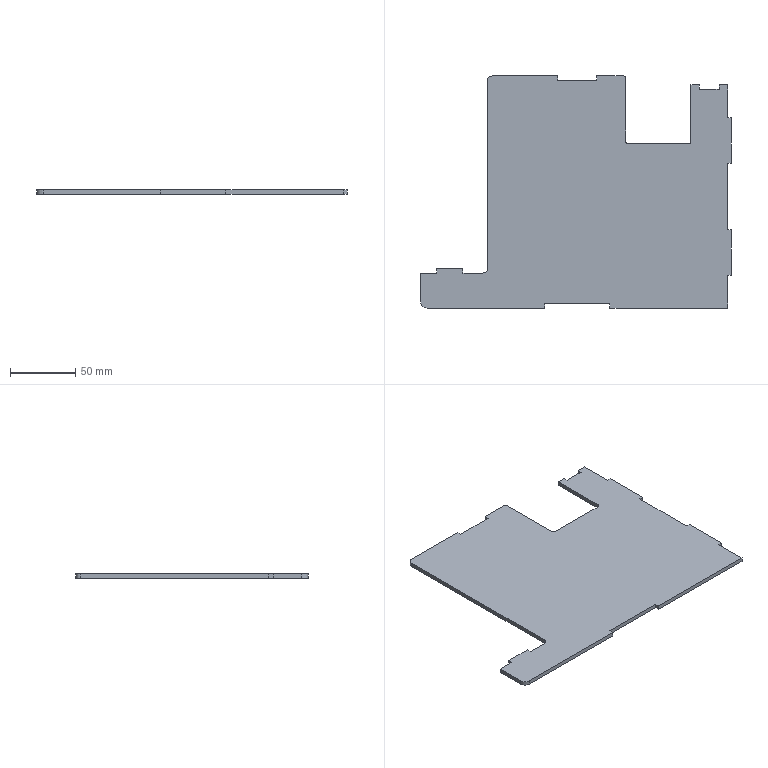Part | SolidWorks | features FlatPattern 1, SMBaseFlange 1, SheetMetal 1 | 1 solid | 42 faces | box 238 x 177.7 x 3.2 mm | volume 99826 mm3 | plane 36 | cylinder 6 | commonest cylinder face diameters 4 x3 7 x2 10 x1
STEP:
#1=CARTESIAN_POINT('',(12.5,-5.5,0.));
#2=VERTEX_POINT('',#1);
#3=CARTESIAN_POINT('',(0.,-5.5,0.));
#4=VERTEX_POINT('',#3);
#5=CARTESIAN_POINT('',(12.5,-5.5,0.));
#6=DIRECTION('',(-1.,0.,0.));
#7=VECTOR('',#6,1000.);
#8=LINE('',#5,#7);
#9=EDGE_CURVE('',#2,#4,#8,.T.);
#10=ORIENTED_EDGE('',*,*,#9,.F.);
#11=CARTESIAN_POINT('',(12.5,-5.5,-3.2));
#12=VERTEX_POINT('',#11);
#13=CARTESIAN_POINT('',(12.5,-5.5,-3.2));
#14=DIRECTION('',(0.,0.,1.));
#15=VECTOR('',#14,1000.);
#16=LINE('',#13,#15);
#17=EDGE_CURVE('',#12,#2,#16,.T.);
#18=ORIENTED_EDGE('',*,*,#17,.F.);
#19=CARTESIAN_POINT('',(0.,-5.5,-3.2));
#20=VERTEX_POINT('',#19);
#21=CARTESIAN_POINT('',(12.5,-5.5,-3.2));
#22=DIRECTION('',(-1.,0.,0.));
#23=VECTOR('',#22,1000.);
#24=LINE('',#21,#23);
#25=EDGE_CURVE('',#12,#20,#24,.T.);
#26=ORIENTED_EDGE('',*,*,#25,.T.);
#27=CARTESIAN_POINT('',(0.,-5.5,-3.2));
#28=DIRECTION('',(0.,0.,1.));
#29=VECTOR('',#28,1000.);
#30=LINE('',#27,#29);
#31=EDGE_CURVE('',#20,#4,#30,.T.);
#32=ORIENTED_EDGE('',*,*,#31,.T.);
#33=EDGE_LOOP('',(#10,#18,#26,#32));
#34=FACE_OUTER_BOUND('',#33,.T.);
#35=CARTESIAN_POINT('',(12.5,-5.5,-3.2));
#36=DIRECTION('',(0.,1.,0.));
#37=DIRECTION('',(-1.,0.,0.));
#38=AXIS2_PLACEMENT_3D('',#35,#36,#37);
#39=PLANE('',#38);
#40=ADVANCED_FACE('',(#34),#39,.T.);
#41=CARTESIAN_POINT('',(12.5,-2.3,0.));
#42=VERTEX_POINT('',#41);
#43=CARTESIAN_POINT('',(12.5,-5.5,0.));
#44=DIRECTION('',(0.,-1.,0.));
#45=VECTOR('',#44,1000.);
#46=LINE('',#43,#45);
#47=EDGE_CURVE('',#42,#2,#46,.T.);
#48=ORIENTED_EDGE('',*,*,#47,.F.);
#49=CARTESIAN_POINT('',(12.5,-2.3,-3.2));
#50=VERTEX_POINT('',#49);
#51=CARTESIAN_POINT('',(12.5,-2.3,-3.2));
#52=DIRECTION('',(0.,0.,1.));
#53=VECTOR('',#52,1000.);
#54=LINE('',#51,#53);
#55=EDGE_CURVE('',#50,#42,#54,.T.);
#56=ORIENTED_EDGE('',*,*,#55,.F.);
#57=CARTESIAN_POINT('',(12.5,-5.5,-3.2));
#58=DIRECTION('',(0.,-1.,0.));
#59=VECTOR('',#58,1000.);
#60=LINE('',#57,#59);
#61=EDGE_CURVE('',#50,#12,#60,.T.);
#62=ORIENTED_EDGE('',*,*,#61,.T.);
#63=ORIENTED_EDGE('',*,*,#17,.T.);
#64=EDGE_LOOP('',(#48,#56,#62,#63));
#65=FACE_OUTER_BOUND('',#64,.T.);
#66=CARTESIAN_POINT('',(12.5,-5.5,-3.2));
#67=DIRECTION('',(-1.,0.,0.));
#68=DIRECTION('',(0.,0.,1.));
#69=AXIS2_PLACEMENT_3D('',#66,#67,#68);
#70=PLANE('',#69);
#71=ADVANCED_FACE('',(#65),#70,.T.);
#72=CARTESIAN_POINT('',(32.5,-2.3,0.));
#73=VERTEX_POINT('',#72);
#74=CARTESIAN_POINT('',(12.5,-2.3,0.));
#75=DIRECTION('',(-1.,0.,0.));
#76=VECTOR('',#75,1000.);
#77=LINE('',#74,#76);
#78=EDGE_CURVE('',#73,#42,#77,.T.);
#79=ORIENTED_EDGE('',*,*,#78,.F.);
#80=CARTESIAN_POINT('',(32.5,-2.3,-3.2));
#81=VERTEX_POINT('',#80);
#82=CARTESIAN_POINT('',(32.5,-2.3,-3.2));
#83=DIRECTION('',(0.,0.,1.));
#84=VECTOR('',#83,1000.);
#85=LINE('',#82,#84);
#86=EDGE_CURVE('',#81,#73,#85,.T.);
#87=ORIENTED_EDGE('',*,*,#86,.F.);
#88=CARTESIAN_POINT('',(12.5,-2.3,-3.2));
#89=DIRECTION('',(-1.,0.,0.));
#90=VECTOR('',#89,1000.);
#91=LINE('',#88,#90);
#92=EDGE_CURVE('',#81,#50,#91,.T.);
#93=ORIENTED_EDGE('',*,*,#92,.T.);
#94=ORIENTED_EDGE('',*,*,#55,.T.);
#95=EDGE_LOOP('',(#79,#87,#93,#94));
#96=FACE_OUTER_BOUND('',#95,.T.);
#97=CARTESIAN_POINT('',(12.5,-2.3,-3.2));
#98=DIRECTION('',(0.,1.,0.));
#99=DIRECTION('',(0.,0.,1.));
#100=AXIS2_PLACEMENT_3D('',#97,#98,#99);
#101=PLANE('',#100);
#102=ADVANCED_FACE('',(#96),#101,.T.);
#103=CARTESIAN_POINT('',(32.5,-5.5,0.));
#104=VERTEX_POINT('',#103);
#105=CARTESIAN_POINT('',(32.5,-2.3,0.));
#106=DIRECTION('',(0.,1.,0.));
#107=VECTOR('',#106,1000.);
#108=LINE('',#105,#107);
#109=EDGE_CURVE('',#104,#73,#108,.T.);
#110=ORIENTED_EDGE('',*,*,#109,.F.);
#111=CARTESIAN_POINT('',(32.5,-5.5,-3.2));
#112=VERTEX_POINT('',#111);
#113=CARTESIAN_POINT('',(32.5,-5.5,-3.2));
#114=DIRECTION('',(0.,0.,1.));
#115=VECTOR('',#114,1000.);
#116=LINE('',#113,#115);
#117=EDGE_CURVE('',#112,#104,#116,.T.);
#118=ORIENTED_EDGE('',*,*,#117,.F.);
#119=CARTESIAN_POINT('',(32.5,-2.3,-3.2));
#120=DIRECTION('',(0.,1.,0.));
#121=VECTOR('',#120,1000.);
#122=LINE('',#119,#121);
#123=EDGE_CURVE('',#112,#81,#122,.T.);
#124=ORIENTED_EDGE('',*,*,#123,.T.);
#125=ORIENTED_EDGE('',*,*,#86,.T.);
#126=EDGE_LOOP('',(#110,#118,#124,#125));
#127=FACE_OUTER_BOUND('',#126,.T.);
#128=CARTESIAN_POINT('',(32.5,-2.3,-3.2));
#129=DIRECTION('',(1.,0.,0.));
#130=DIRECTION('',(0.,0.,-1.));
#131=AXIS2_PLACEMENT_3D('',#128,#129,#130);
#132=PLANE('',#131);
#133=ADVANCED_FACE('',(#127),#132,.T.);
#134=CARTESIAN_POINT('',(47.8,-5.5,0.));
#135=VERTEX_POINT('',#134);
#136=CARTESIAN_POINT('',(47.8,-5.5,0.));
#137=DIRECTION('',(-1.,0.,0.));
#138=VECTOR('',#137,1000.);
#139=LINE('',#136,#138);
#140=EDGE_CURVE('',#135,#104,#139,.T.);
#141=ORIENTED_EDGE('',*,*,#140,.F.);
#142=CARTESIAN_POINT('',(47.8,-5.5,-3.2));
#143=VERTEX_POINT('',#142);
#144=CARTESIAN_POINT('',(47.8,-5.5,-3.2));
#145=DIRECTION('',(0.,0.,1.));
#146=VECTOR('',#145,1000.);
#147=LINE('',#144,#146);
#148=EDGE_CURVE('',#143,#135,#147,.T.);
#149=ORIENTED_EDGE('',*,*,#148,.F.);
#150=CARTESIAN_POINT('',(47.8,-5.5,-3.2));
#151=DIRECTION('',(-1.,0.,0.));
#152=VECTOR('',#151,1000.);
#153=LINE('',#150,#152);
#154=EDGE_CURVE('',#143,#112,#153,.T.);
#155=ORIENTED_EDGE('',*,*,#154,.T.);
#156=ORIENTED_EDGE('',*,*,#117,.T.);
#157=EDGE_LOOP('',(#141,#149,#155,#156));
#158=FACE_OUTER_BOUND('',#157,.T.);
#159=CARTESIAN_POINT('',(47.8,-5.5,-3.2));
#160=DIRECTION('',(0.,1.,0.));
#161=DIRECTION('',(-1.,0.,0.));
#162=AXIS2_PLACEMENT_3D('',#159,#160,#161);
#163=PLANE('',#162);
#164=ADVANCED_FACE('',(#158),#163,.T.);
#165=CARTESIAN_POINT('',(51.3,-2.,0.));
#166=VERTEX_POINT('',#165);
#167=CARTESIAN_POINT('',(47.8,-2.,0.));
#168=DIRECTION('',(0.,0.,-1.));
#169=DIRECTION('',(1.,0.,0.));
#170=AXIS2_PLACEMENT_3D('',#167,#168,#169);
#171=CIRCLE('',#170,3.5);
#172=EDGE_CURVE('',#166,#135,#171,.T.);
#173=ORIENTED_EDGE('',*,*,#172,.F.);
#174=CARTESIAN_POINT('',(51.3,-2.,-3.2));
#175=VERTEX_POINT('',#174);
#176=CARTESIAN_POINT('',(51.3,-2.,-3.2));
#177=DIRECTION('',(0.,0.,1.));
#178=VECTOR('',#177,1000.);
#179=LINE('',#176,#178);
#180=EDGE_CURVE('',#175,#166,#179,.T.);
#181=ORIENTED_EDGE('',*,*,#180,.F.);
#182=CARTESIAN_POINT('',(47.8,-2.,-3.2));
#183=DIRECTION('',(0.,0.,-1.));
#184=DIRECTION('',(1.,0.,0.));
#185=AXIS2_PLACEMENT_3D('',#182,#183,#184);
#186=CIRCLE('',#185,3.5);
#187=EDGE_CURVE('',#175,#143,#186,.T.);
#188=ORIENTED_EDGE('',*,*,#187,.T.);
#189=ORIENTED_EDGE('',*,*,#148,.T.);
#190=EDGE_LOOP('',(#173,#181,#188,#189));
#191=FACE_OUTER_BOUND('',#190,.T.);
#192=CARTESIAN_POINT('',(47.8,-2.,-3.2));
#193=DIRECTION('',(0.,0.,1.));
#194=DIRECTION('',(1.,0.,0.));
#195=AXIS2_PLACEMENT_3D('',#192,#193,#194);
#196=CYLINDRICAL_SURFACE('',#195,3.5);
#197=ADVANCED_FACE('',(#191),#196,.F.);
#198=CARTESIAN_POINT('',(51.3,141.9,0.));
#199=VERTEX_POINT('',#198);
#200=CARTESIAN_POINT('',(51.3,-2.,0.));
#201=DIRECTION('',(0.,-1.,0.));
#202=VECTOR('',#201,1000.);
#203=LINE('',#200,#202);
#204=EDGE_CURVE('',#199,#166,#203,.T.);
#205=ORIENTED_EDGE('',*,*,#204,.F.);
#206=CARTESIAN_POINT('',(51.3,141.9,-3.2));
#207=VERTEX_POINT('',#206);
#208=CARTESIAN_POINT('',(51.3,141.9,-3.2));
#209=DIRECTION('',(0.,0.,1.));
#210=VECTOR('',#209,1000.);
#211=LINE('',#208,#210);
#212=EDGE_CURVE('',#207,#199,#211,.T.);
#213=ORIENTED_EDGE('',*,*,#212,.F.);
#214=CARTESIAN_POINT('',(51.3,-2.,-3.2));
#215=DIRECTION('',(0.,-1.,0.));
#216=VECTOR('',#215,1000.);
#217=LINE('',#214,#216);
#218=EDGE_CURVE('',#207,#175,#217,.T.);
#219=ORIENTED_EDGE('',*,*,#218,.T.);
#220=ORIENTED_EDGE('',*,*,#180,.T.);
#221=EDGE_LOOP('',(#205,#213,#219,#220));
#222=FACE_OUTER_BOUND('',#221,.T.);
#223=CARTESIAN_POINT('',(51.3,-2.,-3.2));
#224=DIRECTION('',(-1.,0.,0.));
#225=DIRECTION('',(0.,-1.,0.));
#226=AXIS2_PLACEMENT_3D('',#223,#224,#225);
#227=PLANE('',#226);
#228=ADVANCED_FACE('',(#222),#227,.T.);
#229=CARTESIAN_POINT('',(54.8,145.4,0.));
#230=VERTEX_POINT('',#229);
#231=CARTESIAN_POINT('',(54.8,141.9,0.));
#232=DIRECTION('',(0.,0.,1.));
#233=DIRECTION('',(1.,0.,0.));
#234=AXIS2_PLACEMENT_3D('',#231,#232,#233);
#235=CIRCLE('',#234,3.5);
#236=EDGE_CURVE('',#230,#199,#235,.T.);
#237=ORIENTED_EDGE('',*,*,#236,.F.);
#238=CARTESIAN_POINT('',(54.8,145.4,-3.2));
#239=VERTEX_POINT('',#238);
#240=CARTESIAN_POINT('',(54.8,145.4,-3.2));
#241=DIRECTION('',(0.,0.,1.));
#242=VECTOR('',#241,1000.);
#243=LINE('',#240,#242);
#244=EDGE_CURVE('',#239,#230,#243,.T.);
#245=ORIENTED_EDGE('',*,*,#244,.F.);
#246=CARTESIAN_POINT('',(54.8,141.9,-3.2));
#247=DIRECTION('',(0.,0.,1.));
#248=DIRECTION('',(1.,0.,0.));
#249=AXIS2_PLACEMENT_3D('',#246,#247,#248);
#250=CIRCLE('',#249,3.5);
#251=EDGE_CURVE('',#239,#207,#250,.T.);
#252=ORIENTED_EDGE('',*,*,#251,.T.);
#253=ORIENTED_EDGE('',*,*,#212,.T.);
#254=EDGE_LOOP('',(#237,#245,#252,#253));
#255=FACE_OUTER_BOUND('',#254,.T.);
#256=CARTESIAN_POINT('',(54.8,141.9,-3.2));
#257=DIRECTION('',(0.,0.,1.));
#258=DIRECTION('',(1.,0.,0.));
#259=AXIS2_PLACEMENT_3D('',#256,#257,#258);
#260=CYLINDRICAL_SURFACE('',#259,3.5);
#261=ADVANCED_FACE('',(#255),#260,.T.);
#262=CARTESIAN_POINT('',(105.,145.4,0.));
#263=VERTEX_POINT('',#262);
#264=CARTESIAN_POINT('',(54.8,145.4,0.));
#265=DIRECTION('',(-1.,0.,0.));
#266=VECTOR('',#265,1000.);
#267=LINE('',#264,#266);
#268=EDGE_CURVE('',#263,#230,#267,.T.);
#269=ORIENTED_EDGE('',*,*,#268,.F.);
#270=CARTESIAN_POINT('',(105.,145.4,-3.2));
#271=VERTEX_POINT('',#270);
#272=CARTESIAN_POINT('',(105.,145.4,-3.2));
#273=DIRECTION('',(0.,0.,1.));
#274=VECTOR('',#273,1000.);
#275=LINE('',#272,#274);
#276=EDGE_CURVE('',#271,#263,#275,.T.);
#277=ORIENTED_EDGE('',*,*,#276,.F.);
#278=CARTESIAN_POINT('',(54.8,145.4,-3.2));
#279=DIRECTION('',(-1.,0.,0.));
#280=VECTOR('',#279,1000.);
#281=LINE('',#278,#280);
#282=EDGE_CURVE('',#271,#239,#281,.T.);
#283=ORIENTED_EDGE('',*,*,#282,.T.);
#284=ORIENTED_EDGE('',*,*,#244,.T.);
#285=EDGE_LOOP('',(#269,#277,#283,#284));
#286=FACE_OUTER_BOUND('',#285,.T.);
#287=CARTESIAN_POINT('',(54.8,145.4,-3.2));
#288=DIRECTION('',(0.,1.,0.));
#289=DIRECTION('',(-1.,0.,0.));
#290=AXIS2_PLACEMENT_3D('',#287,#288,#289);
#291=PLANE('',#290);
#292=ADVANCED_FACE('',(#286),#291,.T.);
#293=CARTESIAN_POINT('',(105.,142.2,0.));
#294=VERTEX_POINT('',#293);
#295=CARTESIAN_POINT('',(105.,145.4,0.));
#296=DIRECTION('',(0.,1.,0.));
#297=VECTOR('',#296,1000.);
#298=LINE('',#295,#297);
#299=EDGE_CURVE('',#294,#263,#298,.T.);
#300=ORIENTED_EDGE('',*,*,#299,.F.);
#301=CARTESIAN_POINT('',(105.,142.2,-3.2));
#302=VERTEX_POINT('',#301);
#303=CARTESIAN_POINT('',(105.,142.2,-3.2));
#304=DIRECTION('',(0.,0.,1.));
#305=VECTOR('',#304,1000.);
#306=LINE('',#303,#305);
#307=EDGE_CURVE('',#302,#294,#306,.T.);
#308=ORIENTED_EDGE('',*,*,#307,.F.);
#309=CARTESIAN_POINT('',(105.,145.4,-3.2));
#310=DIRECTION('',(0.,1.,0.));
#311=VECTOR('',#310,1000.);
#312=LINE('',#309,#311);
#313=EDGE_CURVE('',#302,#271,#312,.T.);
#314=ORIENTED_EDGE('',*,*,#313,.T.);
#315=ORIENTED_EDGE('',*,*,#276,.T.);
#316=EDGE_LOOP('',(#300,#308,#314,#315));
#317=FACE_OUTER_BOUND('',#316,.T.);
#318=CARTESIAN_POINT('',(105.,145.4,-3.2));
#319=DIRECTION('',(1.,0.,0.));
#320=DIRECTION('',(0.,1.,0.));
#321=AXIS2_PLACEMENT_3D('',#318,#319,#320);
#322=PLANE('',#321);
#323=ADVANCED_FACE('',(#317),#322,.T.);
#324=CARTESIAN_POINT('',(135.,142.2,0.));
#325=VERTEX_POINT('',#324);
#326=CARTESIAN_POINT('',(105.,142.2,0.));
#327=DIRECTION('',(-1.,0.,0.));
#328=VECTOR('',#327,1000.);
#329=LINE('',#326,#328);
#330=EDGE_CURVE('',#325,#294,#329,.T.);
#331=ORIENTED_EDGE('',*,*,#330,.F.);
#332=CARTESIAN_POINT('',(135.,142.2,-3.2));
#333=VERTEX_POINT('',#332);
#334=CARTESIAN_POINT('',(135.,142.2,-3.2));
#335=DIRECTION('',(0.,0.,1.));
#336=VECTOR('',#335,1000.);
#337=LINE('',#334,#336);
#338=EDGE_CURVE('',#333,#325,#337,.T.);
#339=ORIENTED_EDGE('',*,*,#338,.F.);
#340=CARTESIAN_POINT('',(105.,142.2,-3.2));
#341=DIRECTION('',(-1.,0.,0.));
#342=VECTOR('',#341,1000.);
#343=LINE('',#340,#342);
#344=EDGE_CURVE('',#333,#302,#343,.T.);
#345=ORIENTED_EDGE('',*,*,#344,.T.);
#346=ORIENTED_EDGE('',*,*,#307,.T.);
#347=EDGE_LOOP('',(#331,#339,#345,#346));
#348=FACE_OUTER_BOUND('',#347,.T.);
#349=CARTESIAN_POINT('',(105.,142.2,-3.2));
#350=DIRECTION('',(0.,1.,0.));
#351=DIRECTION('',(-1.,0.,0.));
#352=AXIS2_PLACEMENT_3D('',#349,#350,#351);
#353=PLANE('',#352);
#354=ADVANCED_FACE('',(#348),#353,.T.);
#355=CARTESIAN_POINT('',(135.,145.4,0.));
#356=VERTEX_POINT('',#355);
#357=CARTESIAN_POINT('',(135.,142.2,0.));
#358=DIRECTION('',(0.,-1.,0.));
#359=VECTOR('',#358,1000.);
#360=LINE('',#357,#359);
#361=EDGE_CURVE('',#356,#325,#360,.T.);
#362=ORIENTED_EDGE('',*,*,#361,.F.);
#363=CARTESIAN_POINT('',(135.,145.4,-3.2));
#364=VERTEX_POINT('',#363);
#365=CARTESIAN_POINT('',(135.,145.4,-3.2));
#366=DIRECTION('',(0.,0.,1.));
#367=VECTOR('',#366,1000.);
#368=LINE('',#365,#367);
#369=EDGE_CURVE('',#364,#356,#368,.T.);
#370=ORIENTED_EDGE('',*,*,#369,.F.);
#371=CARTESIAN_POINT('',(135.,142.2,-3.2));
#372=DIRECTION('',(0.,-1.,0.));
#373=VECTOR('',#372,1000.);
#374=LINE('',#371,#373);
#375=EDGE_CURVE('',#364,#333,#374,.T.);
#376=ORIENTED_EDGE('',*,*,#375,.T.);
#377=ORIENTED_EDGE('',*,*,#338,.T.);
#378=EDGE_LOOP('',(#362,#370,#376,#377));
#379=FACE_OUTER_BOUND('',#378,.T.);
#380=CARTESIAN_POINT('',(135.,142.2,-3.2));
#381=DIRECTION('',(-1.,0.,0.));
#382=DIRECTION('',(0.,0.,1.));
#383=AXIS2_PLACEMENT_3D('',#380,#381,#382);
#384=PLANE('',#383);
#385=ADVANCED_FACE('',(#379),#384,.T.);
#386=CARTESIAN_POINT('',(155.,145.4,0.));
#387=VERTEX_POINT('',#386);
#388=CARTESIAN_POINT('',(135.,145.4,0.));
#389=DIRECTION('',(-1.,0.,0.));
#390=VECTOR('',#389,1000.);
#391=LINE('',#388,#390);
#392=EDGE_CURVE('',#387,#356,#391,.T.);
#393=ORIENTED_EDGE('',*,*,#392,.F.);
#394=CARTESIAN_POINT('',(155.,145.4,-3.2));
#395=VERTEX_POINT('',#394);
#396=CARTESIAN_POINT('',(155.,145.4,-3.2));
#397=DIRECTION('',(0.,0.,1.));
#398=VECTOR('',#397,1000.);
#399=LINE('',#396,#398);
#400=EDGE_CURVE('',#395,#387,#399,.T.);
#401=ORIENTED_EDGE('',*,*,#400,.F.);
#402=CARTESIAN_POINT('',(135.,145.4,-3.2));
#403=DIRECTION('',(-1.,0.,0.));
#404=VECTOR('',#403,1000.);
#405=LINE('',#402,#404);
#406=EDGE_CURVE('',#395,#364,#405,.T.);
#407=ORIENTED_EDGE('',*,*,#406,.T.);
#408=ORIENTED_EDGE('',*,*,#369,.T.);
#409=EDGE_LOOP('',(#393,#401,#407,#408));
#410=FACE_OUTER_BOUND('',#409,.T.);
#411=CARTESIAN_POINT('',(135.,145.4,-3.2));
#412=DIRECTION('',(0.,1.,0.));
#413=DIRECTION('',(-1.,0.,0.));
#414=AXIS2_PLACEMENT_3D('',#411,#412,#413);
#415=PLANE('',#414);
#416=ADVANCED_FACE('',(#410),#415,.T.);
#417=CARTESIAN_POINT('',(157.,143.4,0.));
#418=VERTEX_POINT('',#417);
#419=CARTESIAN_POINT('',(155.,143.4,0.));
#420=DIRECTION('',(0.,0.,1.));
#421=DIRECTION('',(-1.,0.,0.));
#422=AXIS2_PLACEMENT_3D('',#419,#420,#421);
#423=CIRCLE('',#422,2.);
#424=EDGE_CURVE('',#418,#387,#423,.T.);
#425=ORIENTED_EDGE('',*,*,#424,.F.);
#426=CARTESIAN_POINT('',(157.,143.4,-3.2));
#427=VERTEX_POINT('',#426);
#428=CARTESIAN_POINT('',(157.,143.4,-3.2));
#429=DIRECTION('',(0.,0.,1.));
#430=VECTOR('',#429,1000.);
#431=LINE('',#428,#430);
#432=EDGE_CURVE('',#427,#418,#431,.T.);
#433=ORIENTED_EDGE('',*,*,#432,.F.);
#434=CARTESIAN_POINT('',(155.,143.4,-3.2));
#435=DIRECTION('',(0.,0.,1.));
#436=DIRECTION('',(-1.,0.,0.));
#437=AXIS2_PLACEMENT_3D('',#434,#435,#436);
#438=CIRCLE('',#437,2.);
#439=EDGE_CURVE('',#427,#395,#438,.T.);
#440=ORIENTED_EDGE('',*,*,#439,.T.);
#441=ORIENTED_EDGE('',*,*,#400,.T.);
#442=EDGE_LOOP('',(#425,#433,#440,#441));
#443=FACE_OUTER_BOUND('',#442,.T.);
#444=CARTESIAN_POINT('',(155.,143.4,-3.2));
#445=DIRECTION('',(0.,0.,1.));
#446=DIRECTION('',(1.,0.,0.));
#447=AXIS2_PLACEMENT_3D('',#444,#445,#446);
#448=CYLINDRICAL_SURFACE('',#447,2.);
#449=ADVANCED_FACE('',(#443),#448,.T.);
#450=CARTESIAN_POINT('',(157.,95.5,0.));
#451=VERTEX_POINT('',#450);
#452=CARTESIAN_POINT('',(157.,95.5,0.));
#453=DIRECTION('',(0.,1.,0.));
#454=VECTOR('',#453,1000.);
#455=LINE('',#452,#454);
#456=EDGE_CURVE('',#451,#418,#455,.T.);
#457=ORIENTED_EDGE('',*,*,#456,.F.);
#458=CARTESIAN_POINT('',(157.,95.5,-3.2));
#459=VERTEX_POINT('',#458);
#460=CARTESIAN_POINT('',(157.,95.5,-3.2));
#461=DIRECTION('',(0.,0.,1.));
#462=VECTOR('',#461,1000.);
#463=LINE('',#460,#462);
#464=EDGE_CURVE('',#459,#451,#463,.T.);
#465=ORIENTED_EDGE('',*,*,#464,.F.);
#466=CARTESIAN_POINT('',(157.,95.5,-3.2));
#467=DIRECTION('',(0.,1.,0.));
#468=VECTOR('',#467,1000.);
#469=LINE('',#466,#468);
#470=EDGE_CURVE('',#459,#427,#469,.T.);
#471=ORIENTED_EDGE('',*,*,#470,.T.);
#472=ORIENTED_EDGE('',*,*,#432,.T.);
#473=EDGE_LOOP('',(#457,#465,#471,#472));
#474=FACE_OUTER_BOUND('',#473,.T.);
#475=CARTESIAN_POINT('',(157.,95.5,-3.2));
#476=DIRECTION('',(1.,0.,0.));
#477=DIRECTION('',(0.,0.,-1.));
#478=AXIS2_PLACEMENT_3D('',#475,#476,#477);
#479=PLANE('',#478);
#480=ADVANCED_FACE('',(#474),#479,.T.);
#481=CARTESIAN_POINT('',(159.,93.5,0.));
#482=VERTEX_POINT('',#481);
#483=CARTESIAN_POINT('',(159.,95.5,0.));
#484=DIRECTION('',(0.,0.,-1.));
#485=DIRECTION('',(-1.,0.,0.));
#486=AXIS2_PLACEMENT_3D('',#483,#484,#485);
#487=CIRCLE('',#486,2.);
#488=EDGE_CURVE('',#482,#451,#487,.T.);
#489=ORIENTED_EDGE('',*,*,#488,.F.);
#490=CARTESIAN_POINT('',(159.,93.5,-3.2));
#491=VERTEX_POINT('',#490);
#492=CARTESIAN_POINT('',(159.,93.5,-3.2));
#493=DIRECTION('',(0.,0.,1.));
#494=VECTOR('',#493,1000.);
#495=LINE('',#492,#494);
#496=EDGE_CURVE('',#491,#482,#495,.T.);
#497=ORIENTED_EDGE('',*,*,#496,.F.);
#498=CARTESIAN_POINT('',(159.,95.5,-3.2));
#499=DIRECTION('',(0.,0.,-1.));
#500=DIRECTION('',(-1.,0.,0.));
#501=AXIS2_PLACEMENT_3D('',#498,#499,#500);
#502=CIRCLE('',#501,2.);
#503=EDGE_CURVE('',#491,#459,#502,.T.);
#504=ORIENTED_EDGE('',*,*,#503,.T.);
#505=ORIENTED_EDGE('',*,*,#464,.T.);
#506=EDGE_LOOP('',(#489,#497,#504,#505));
#507=FACE_OUTER_BOUND('',#506,.T.);
#508=CARTESIAN_POINT('',(159.,95.5,-3.2));
#509=DIRECTION('',(0.,0.,1.));
#510=DIRECTION('',(1.,0.,0.));
#511=AXIS2_PLACEMENT_3D('',#508,#509,#510);
#512=CYLINDRICAL_SURFACE('',#511,2.);
#513=ADVANCED_FACE('',(#507),#512,.F.);
#514=CARTESIAN_POINT('',(205.,93.5,0.));
#515=VERTEX_POINT('',#514);
#516=CARTESIAN_POINT('',(205.,93.5,0.));
#517=DIRECTION('',(-1.,0.,0.));
#518=VECTOR('',#517,1000.);
#519=LINE('',#516,#518);
#520=EDGE_CURVE('',#515,#482,#519,.T.);
#521=ORIENTED_EDGE('',*,*,#520,.F.);
#522=CARTESIAN_POINT('',(205.,93.5,-3.2));
#523=VERTEX_POINT('',#522);
#524=CARTESIAN_POINT('',(205.,93.5,-3.2));
#525=DIRECTION('',(0.,0.,1.));
#526=VECTOR('',#525,1000.);
#527=LINE('',#524,#526);
#528=EDGE_CURVE('',#523,#515,#527,.T.);
#529=ORIENTED_EDGE('',*,*,#528,.F.);
#530=CARTESIAN_POINT('',(205.,93.5,-3.2));
#531=DIRECTION('',(-1.,0.,0.));
#532=VECTOR('',#531,1000.);
#533=LINE('',#530,#532);
#534=EDGE_CURVE('',#523,#491,#533,.T.);
#535=ORIENTED_EDGE('',*,*,#534,.T.);
#536=ORIENTED_EDGE('',*,*,#496,.T.);
#537=EDGE_LOOP('',(#521,#529,#535,#536));
#538=FACE_OUTER_BOUND('',#537,.T.);
#539=CARTESIAN_POINT('',(205.,93.5,-3.2));
#540=DIRECTION('',(0.,1.,0.));
#541=DIRECTION('',(-1.,0.,0.));
#542=AXIS2_PLACEMENT_3D('',#539,#540,#541);
#543=PLANE('',#542);
#544=ADVANCED_FACE('',(#538),#543,.T.);
#545=CARTESIAN_POINT('',(207.,95.5,0.));
#546=VERTEX_POINT('',#545);
#547=CARTESIAN_POINT('',(205.,95.5,0.));
#548=DIRECTION('',(0.,0.,-1.));
#549=DIRECTION('',(-1.,0.,0.));
#550=AXIS2_PLACEMENT_3D('',#547,#548,#549);
#551=CIRCLE('',#550,2.);
#552=EDGE_CURVE('',#546,#515,#551,.T.);
#553=ORIENTED_EDGE('',*,*,#552,.F.);
#554=CARTESIAN_POINT('',(207.,95.5,-3.2));
#555=VERTEX_POINT('',#554);
#556=CARTESIAN_POINT('',(207.,95.5,-3.2));
#557=DIRECTION('',(0.,0.,1.));
#558=VECTOR('',#557,1000.);
#559=LINE('',#556,#558);
#560=EDGE_CURVE('',#555,#546,#559,.T.);
#561=ORIENTED_EDGE('',*,*,#560,.F.);
#562=CARTESIAN_POINT('',(205.,95.5,-3.2));
#563=DIRECTION('',(0.,0.,-1.));
#564=DIRECTION('',(-1.,0.,0.));
#565=AXIS2_PLACEMENT_3D('',#562,#563,#564);
#566=CIRCLE('',#565,2.);
#567=EDGE_CURVE('',#555,#523,#566,.T.);
#568=ORIENTED_EDGE('',*,*,#567,.T.);
#569=ORIENTED_EDGE('',*,*,#528,.T.);
#570=EDGE_LOOP('',(#553,#561,#568,#569));
#571=FACE_OUTER_BOUND('',#570,.T.);
#572=CARTESIAN_POINT('',(205.,95.5,-3.2));
#573=DIRECTION('',(0.,0.,1.));
#574=DIRECTION('',(1.,0.,0.));
#575=AXIS2_PLACEMENT_3D('',#572,#573,#574);
#576=CYLINDRICAL_SURFACE('',#575,2.);
#577=ADVANCED_FACE('',(#571),#576,.F.);
#578=CARTESIAN_POINT('',(207.,138.5,0.));
#579=VERTEX_POINT('',#578);
#580=CARTESIAN_POINT('',(207.,138.5,0.));
#581=DIRECTION('',(0.,-1.,0.));
#582=VECTOR('',#581,1000.);
#583=LINE('',#580,#582);
#584=EDGE_CURVE('',#579,#546,#583,.T.);
#585=ORIENTED_EDGE('',*,*,#584,.F.);
#586=CARTESIAN_POINT('',(207.,138.5,-3.2));
#587=VERTEX_POINT('',#586);
#588=CARTESIAN_POINT('',(207.,138.5,-3.2));
#589=DIRECTION('',(0.,0.,1.));
#590=VECTOR('',#589,1000.);
#591=LINE('',#588,#590);
#592=EDGE_CURVE('',#587,#579,#591,.T.);
#593=ORIENTED_EDGE('',*,*,#592,.F.);
#594=CARTESIAN_POINT('',(207.,138.5,-3.2));
#595=DIRECTION('',(0.,-1.,0.));
#596=VECTOR('',#595,1000.);
#597=LINE('',#594,#596);
#598=EDGE_CURVE('',#587,#555,#597,.T.);
#599=ORIENTED_EDGE('',*,*,#598,.T.);
#600=ORIENTED_EDGE('',*,*,#560,.T.);
#601=EDGE_LOOP('',(#585,#593,#599,#600));
#602=FACE_OUTER_BOUND('',#601,.T.);
#603=CARTESIAN_POINT('',(207.,138.5,-3.2));
#604=DIRECTION('',(-1.,0.,0.));
#605=DIRECTION('',(0.,-1.,0.));
#606=AXIS2_PLACEMENT_3D('',#603,#604,#605);
#607=PLANE('',#606);
#608=ADVANCED_FACE('',(#602),#607,.T.);
#609=CARTESIAN_POINT('',(213.5,138.5,0.));
#610=VERTEX_POINT('',#609);
#611=CARTESIAN_POINT('',(213.5,138.5,0.));
#612=DIRECTION('',(-1.,0.,0.));
#613=VECTOR('',#612,1000.);
#614=LINE('',#611,#613);
#615=EDGE_CURVE('',#610,#579,#614,.T.);
#616=ORIENTED_EDGE('',*,*,#615,.F.);
#617=CARTESIAN_POINT('',(213.5,138.5,-3.2));
#618=VERTEX_POINT('',#617);
#619=CARTESIAN_POINT('',(213.5,138.5,-3.2));
#620=DIRECTION('',(0.,0.,1.));
#621=VECTOR('',#620,1000.);
#622=LINE('',#619,#621);
#623=EDGE_CURVE('',#618,#610,#622,.T.);
#624=ORIENTED_EDGE('',*,*,#623,.F.);
#625=CARTESIAN_POINT('',(213.5,138.5,-3.2));
#626=DIRECTION('',(-1.,0.,0.));
#627=VECTOR('',#626,1000.);
#628=LINE('',#625,#627);
#629=EDGE_CURVE('',#618,#587,#628,.T.);
#630=ORIENTED_EDGE('',*,*,#629,.T.);
#631=ORIENTED_EDGE('',*,*,#592,.T.);
#632=EDGE_LOOP('',(#616,#624,#630,#631));
#633=FACE_OUTER_BOUND('',#632,.T.);
#634=CARTESIAN_POINT('',(213.5,138.5,-3.2));
#635=DIRECTION('',(0.,1.,0.));
#636=DIRECTION('',(-1.,0.,0.));
#637=AXIS2_PLACEMENT_3D('',#634,#635,#636);
#638=PLANE('',#637);
#639=ADVANCED_FACE('',(#633),#638,.T.);
#640=CARTESIAN_POINT('',(213.5,135.3,0.));
#641=VERTEX_POINT('',#640);
#642=CARTESIAN_POINT('',(213.5,138.5,0.));
#643=DIRECTION('',(0.,1.,0.));
#644=VECTOR('',#643,1000.);
#645=LINE('',#642,#644);
#646=EDGE_CURVE('',#641,#610,#645,.T.);
#647=ORIENTED_EDGE('',*,*,#646,.F.);
#648=CARTESIAN_POINT('',(213.5,135.3,-3.2));
#649=VERTEX_POINT('',#648);
#650=CARTESIAN_POINT('',(213.5,135.3,-3.2));
#651=DIRECTION('',(0.,0.,1.));
#652=VECTOR('',#651,1000.);
#653=LINE('',#650,#652);
#654=EDGE_CURVE('',#649,#641,#653,.T.);
#655=ORIENTED_EDGE('',*,*,#654,.F.);
#656=CARTESIAN_POINT('',(213.5,138.5,-3.2));
#657=DIRECTION('',(0.,1.,0.));
#658=VECTOR('',#657,1000.);
#659=LINE('',#656,#658);
#660=EDGE_CURVE('',#649,#618,#659,.T.);
#661=ORIENTED_EDGE('',*,*,#660,.T.);
#662=ORIENTED_EDGE('',*,*,#623,.T.);
#663=EDGE_LOOP('',(#647,#655,#661,#662));
#664=FACE_OUTER_BOUND('',#663,.T.);
#665=CARTESIAN_POINT('',(213.5,138.5,-3.2));
#666=DIRECTION('',(1.,0.,0.));
#667=DIRECTION('',(0.,0.,-1.));
#668=AXIS2_PLACEMENT_3D('',#665,#666,#667);
#669=PLANE('',#668);
#670=ADVANCED_FACE('',(#664),#669,.T.);
#671=CARTESIAN_POINT('',(228.5,135.3,0.));
#672=VERTEX_POINT('',#671);
#673=CARTESIAN_POINT('',(213.5,135.3,0.));
#674=DIRECTION('',(-1.,0.,0.));
#675=VECTOR('',#674,1000.);
#676=LINE('',#673,#675);
#677=EDGE_CURVE('',#672,#641,#676,.T.);
#678=ORIENTED_EDGE('',*,*,#677,.F.);
#679=CARTESIAN_POINT('',(228.5,135.3,-3.2));
#680=VERTEX_POINT('',#679);
#681=CARTESIAN_POINT('',(228.5,135.3,-3.2));
#682=DIRECTION('',(0.,0.,1.));
#683=VECTOR('',#682,1000.);
#684=LINE('',#681,#683);
#685=EDGE_CURVE('',#680,#672,#684,.T.);
#686=ORIENTED_EDGE('',*,*,#685,.F.);
#687=CARTESIAN_POINT('',(213.5,135.3,-3.2));
#688=DIRECTION('',(-1.,0.,0.));
#689=VECTOR('',#688,1000.);
#690=LINE('',#687,#689);
#691=EDGE_CURVE('',#680,#649,#690,.T.);
#692=ORIENTED_EDGE('',*,*,#691,.T.);
#693=ORIENTED_EDGE('',*,*,#654,.T.);
#694=EDGE_LOOP('',(#678,#686,#692,#693));
#695=FACE_OUTER_BOUND('',#694,.T.);
#696=CARTESIAN_POINT('',(213.5,135.3,-3.2));
#697=DIRECTION('',(0.,1.,0.));
#698=DIRECTION('',(-1.,0.,0.));
#699=AXIS2_PLACEMENT_3D('',#696,#697,#698);
#700=PLANE('',#699);
#701=ADVANCED_FACE('',(#695),#700,.T.);
#702=CARTESIAN_POINT('',(228.5,138.5,0.));
#703=VERTEX_POINT('',#702);
#704=CARTESIAN_POINT('',(228.5,135.3,0.));
#705=DIRECTION('',(0.,-1.,0.));
#706=VECTOR('',#705,1000.);
#707=LINE('',#704,#706);
#708=EDGE_CURVE('',#703,#672,#707,.T.);
#709=ORIENTED_EDGE('',*,*,#708,.F.);
#710=CARTESIAN_POINT('',(228.5,138.5,-3.2));
#711=VERTEX_POINT('',#710);
#712=CARTESIAN_POINT('',(228.5,138.5,-3.2));
#713=DIRECTION('',(0.,0.,1.));
#714=VECTOR('',#713,1000.);
#715=LINE('',#712,#714);
#716=EDGE_CURVE('',#711,#703,#715,.T.);
#717=ORIENTED_EDGE('',*,*,#716,.F.);
#718=CARTESIAN_POINT('',(228.5,135.3,-3.2));
#719=DIRECTION('',(0.,-1.,0.));
#720=VECTOR('',#719,1000.);
#721=LINE('',#718,#720);
#722=EDGE_CURVE('',#711,#680,#721,.T.);
#723=ORIENTED_EDGE('',*,*,#722,.T.);
#724=ORIENTED_EDGE('',*,*,#685,.T.);
#725=EDGE_LOOP('',(#709,#717,#723,#724));
#726=FACE_OUTER_BOUND('',#725,.T.);
#727=CARTESIAN_POINT('',(228.5,135.3,-3.2));
#728=DIRECTION('',(-1.,0.,0.));
#729=DIRECTION('',(0.,0.,1.));
#730=AXIS2_PLACEMENT_3D('',#727,#728,#729);
#731=PLANE('',#730);
#732=ADVANCED_FACE('',(#726),#731,.T.);
#733=CARTESIAN_POINT('',(235.,138.5,0.));
#734=VERTEX_POINT('',#733);
#735=CARTESIAN_POINT('',(235.,138.5,0.));
#736=DIRECTION('',(-1.,0.,0.));
#737=VECTOR('',#736,1000.);
#738=LINE('',#735,#737);
#739=EDGE_CURVE('',#734,#703,#738,.T.);
#740=ORIENTED_EDGE('',*,*,#739,.F.);
#741=CARTESIAN_POINT('',(235.,138.5,-3.2));
#742=VERTEX_POINT('',#741);
#743=CARTESIAN_POINT('',(235.,138.5,-3.2));
#744=DIRECTION('',(0.,0.,1.));
#745=VECTOR('',#744,1000.);
#746=LINE('',#743,#745);
#747=EDGE_CURVE('',#742,#734,#746,.T.);
#748=ORIENTED_EDGE('',*,*,#747,.F.);
#749=CARTESIAN_POINT('',(235.,138.5,-3.2));
#750=DIRECTION('',(-1.,0.,0.));
#751=VECTOR('',#750,1000.);
#752=LINE('',#749,#751);
#753=EDGE_CURVE('',#742,#711,#752,.T.);
#754=ORIENTED_EDGE('',*,*,#753,.T.);
#755=ORIENTED_EDGE('',*,*,#716,.T.);
#756=EDGE_LOOP('',(#740,#748,#754,#755));
#757=FACE_OUTER_BOUND('',#756,.T.);
#758=CARTESIAN_POINT('',(235.,138.5,-3.2));
#759=DIRECTION('',(0.,1.,0.));
#760=DIRECTION('',(-1.,0.,0.));
#761=AXIS2_PLACEMENT_3D('',#758,#759,#760);
#762=PLANE('',#761);
#763=ADVANCED_FACE('',(#757),#762,.T.);
#764=CARTESIAN_POINT('',(235.,113.5,0.));
#765=VERTEX_POINT('',#764);
#766=CARTESIAN_POINT('',(235.,113.5,0.));
#767=DIRECTION('',(0.,1.,0.));
#768=VECTOR('',#767,1000.);
#769=LINE('',#766,#768);
#770=EDGE_CURVE('',#765,#734,#769,.T.);
#771=ORIENTED_EDGE('',*,*,#770,.F.);
#772=CARTESIAN_POINT('',(235.,113.5,-3.2));
#773=VERTEX_POINT('',#772);
#774=CARTESIAN_POINT('',(235.,113.5,-3.2));
#775=DIRECTION('',(0.,0.,1.));
#776=VECTOR('',#775,1000.);
#777=LINE('',#774,#776);
#778=EDGE_CURVE('',#773,#765,#777,.T.);
#779=ORIENTED_EDGE('',*,*,#778,.F.);
#780=CARTESIAN_POINT('',(235.,113.5,-3.2));
#781=DIRECTION('',(0.,1.,0.));
#782=VECTOR('',#781,1000.);
#783=LINE('',#780,#782);
#784=EDGE_CURVE('',#773,#742,#783,.T.);
#785=ORIENTED_EDGE('',*,*,#784,.T.);
#786=ORIENTED_EDGE('',*,*,#747,.T.);
#787=EDGE_LOOP('',(#771,#779,#785,#786));
#788=FACE_OUTER_BOUND('',#787,.T.);
#789=CARTESIAN_POINT('',(235.,113.5,-3.2));
#790=DIRECTION('',(1.,0.,0.));
#791=DIRECTION('',(0.,0.,-1.));
#792=AXIS2_PLACEMENT_3D('',#789,#790,#791);
#793=PLANE('',#792);
#794=ADVANCED_FACE('',(#788),#793,.T.);
#795=CARTESIAN_POINT('',(238.,113.5,0.));
#796=VERTEX_POINT('',#795);
#797=CARTESIAN_POINT('',(235.,113.5,0.));
#798=DIRECTION('',(-1.,0.,0.));
#799=VECTOR('',#798,1000.);
#800=LINE('',#797,#799);
#801=EDGE_CURVE('',#796,#765,#800,.T.);
#802=ORIENTED_EDGE('',*,*,#801,.F.);
#803=CARTESIAN_POINT('',(238.,113.5,-3.2));
#804=VERTEX_POINT('',#803);
#805=CARTESIAN_POINT('',(238.,113.5,-3.2));
#806=DIRECTION('',(0.,0.,1.));
#807=VECTOR('',#806,1000.);
#808=LINE('',#805,#807);
#809=EDGE_CURVE('',#804,#796,#808,.T.);
#810=ORIENTED_EDGE('',*,*,#809,.F.);
#811=CARTESIAN_POINT('',(235.,113.5,-3.2));
#812=DIRECTION('',(-1.,0.,0.));
#813=VECTOR('',#812,1000.);
#814=LINE('',#811,#813);
#815=EDGE_CURVE('',#804,#773,#814,.T.);
#816=ORIENTED_EDGE('',*,*,#815,.T.);
#817=ORIENTED_EDGE('',*,*,#778,.T.);
#818=EDGE_LOOP('',(#802,#810,#816,#817));
#819=FACE_OUTER_BOUND('',#818,.T.);
#820=CARTESIAN_POINT('',(235.,113.5,-3.2));
#821=DIRECTION('',(0.,1.,0.));
#822=DIRECTION('',(0.,0.,1.));
#823=AXIS2_PLACEMENT_3D('',#820,#821,#822);
#824=PLANE('',#823);
#825=ADVANCED_FACE('',(#819),#824,.T.);
#826=CARTESIAN_POINT('',(238.,78.5,0.));
#827=VERTEX_POINT('',#826);
#828=CARTESIAN_POINT('',(238.,113.5,0.));
#829=DIRECTION('',(0.,1.,0.));
#830=VECTOR('',#829,1000.);
#831=LINE('',#828,#830);
#832=EDGE_CURVE('',#827,#796,#831,.T.);
#833=ORIENTED_EDGE('',*,*,#832,.F.);
#834=CARTESIAN_POINT('',(238.,78.5,-3.2));
#835=VERTEX_POINT('',#834);
#836=CARTESIAN_POINT('',(238.,78.5,-3.2));
#837=DIRECTION('',(0.,0.,1.));
#838=VECTOR('',#837,1000.);
#839=LINE('',#836,#838);
#840=EDGE_CURVE('',#835,#827,#839,.T.);
#841=ORIENTED_EDGE('',*,*,#840,.F.);
#842=CARTESIAN_POINT('',(238.,113.5,-3.2));
#843=DIRECTION('',(0.,1.,0.));
#844=VECTOR('',#843,1000.);
#845=LINE('',#842,#844);
#846=EDGE_CURVE('',#835,#804,#845,.T.);
#847=ORIENTED_EDGE('',*,*,#846,.T.);
#848=ORIENTED_EDGE('',*,*,#809,.T.);
#849=EDGE_LOOP('',(#833,#841,#847,#848));
#850=FACE_OUTER_BOUND('',#849,.T.);
#851=CARTESIAN_POINT('',(238.,113.5,-3.2));
#852=DIRECTION('',(1.,0.,0.));
#853=DIRECTION('',(0.,0.,-1.));
#854=AXIS2_PLACEMENT_3D('',#851,#852,#853);
#855=PLANE('',#854);
#856=ADVANCED_FACE('',(#850),#855,.T.);
#857=CARTESIAN_POINT('',(235.,78.5,0.));
#858=VERTEX_POINT('',#857);
#859=CARTESIAN_POINT('',(238.,78.5,0.));
#860=DIRECTION('',(1.,0.,0.));
#861=VECTOR('',#860,1000.);
#862=LINE('',#859,#861);
#863=EDGE_CURVE('',#858,#827,#862,.T.);
#864=ORIENTED_EDGE('',*,*,#863,.F.);
#865=CARTESIAN_POINT('',(235.,78.5,-3.2));
#866=VERTEX_POINT('',#865);
#867=CARTESIAN_POINT('',(235.,78.5,-3.2));
#868=DIRECTION('',(0.,0.,1.));
#869=VECTOR('',#868,1000.);
#870=LINE('',#867,#869);
#871=EDGE_CURVE('',#866,#858,#870,.T.);
#872=ORIENTED_EDGE('',*,*,#871,.F.);
#873=CARTESIAN_POINT('',(238.,78.5,-3.2));
#874=DIRECTION('',(1.,0.,0.));
#875=VECTOR('',#874,1000.);
#876=LINE('',#873,#875);
#877=EDGE_CURVE('',#866,#835,#876,.T.);
#878=ORIENTED_EDGE('',*,*,#877,.T.);
#879=ORIENTED_EDGE('',*,*,#840,.T.);
#880=EDGE_LOOP('',(#864,#872,#878,#879));
#881=FACE_OUTER_BOUND('',#880,.T.);
#882=CARTESIAN_POINT('',(238.,78.5,-3.2));
#883=DIRECTION('',(0.,-1.,0.));
#884=DIRECTION('',(0.,0.,-1.));
#885=AXIS2_PLACEMENT_3D('',#882,#883,#884);
#886=PLANE('',#885);
#887=ADVANCED_FACE('',(#881),#886,.T.);
#888=CARTESIAN_POINT('',(235.,27.7,0.));
#889=VERTEX_POINT('',#888);
#890=CARTESIAN_POINT('',(235.,27.7,0.));
#891=DIRECTION('',(0.,1.,0.));
#892=VECTOR('',#891,1000.);
#893=LINE('',#890,#892);
#894=EDGE_CURVE('',#889,#858,#893,.T.);
#895=ORIENTED_EDGE('',*,*,#894,.F.);
#896=CARTESIAN_POINT('',(235.,27.7,-3.2));
#897=VERTEX_POINT('',#896);
#898=CARTESIAN_POINT('',(235.,27.7,-3.2));
#899=DIRECTION('',(0.,0.,1.));
#900=VECTOR('',#899,1000.);
#901=LINE('',#898,#900);
#902=EDGE_CURVE('',#897,#889,#901,.T.);
#903=ORIENTED_EDGE('',*,*,#902,.F.);
#904=CARTESIAN_POINT('',(235.,27.7,-3.2));
#905=DIRECTION('',(0.,1.,0.));
#906=VECTOR('',#905,1000.);
#907=LINE('',#904,#906);
#908=EDGE_CURVE('',#897,#866,#907,.T.);
#909=ORIENTED_EDGE('',*,*,#908,.T.);
#910=ORIENTED_EDGE('',*,*,#871,.T.);
#911=EDGE_LOOP('',(#895,#903,#909,#910));
#912=FACE_OUTER_BOUND('',#911,.T.);
#913=CARTESIAN_POINT('',(235.,27.7,-3.2));
#914=DIRECTION('',(1.,0.,0.));
#915=DIRECTION('',(0.,0.,-1.));
#916=AXIS2_PLACEMENT_3D('',#913,#914,#915);
#917=PLANE('',#916);
#918=ADVANCED_FACE('',(#912),#917,.T.);
#919=CARTESIAN_POINT('',(238.,27.7,0.));
#920=VERTEX_POINT('',#919);
#921=CARTESIAN_POINT('',(238.,27.7,0.));
#922=DIRECTION('',(-1.,0.,0.));
#923=VECTOR('',#922,1000.);
#924=LINE('',#921,#923);
#925=EDGE_CURVE('',#920,#889,#924,.T.);
#926=ORIENTED_EDGE('',*,*,#925,.F.);
#927=CARTESIAN_POINT('',(238.,27.7,-3.2));
#928=VERTEX_POINT('',#927);
#929=CARTESIAN_POINT('',(238.,27.7,-3.2));
#930=DIRECTION('',(0.,0.,1.));
#931=VECTOR('',#930,1000.);
#932=LINE('',#929,#931);
#933=EDGE_CURVE('',#928,#920,#932,.T.);
#934=ORIENTED_EDGE('',*,*,#933,.F.);
#935=CARTESIAN_POINT('',(238.,27.7,-3.2));
#936=DIRECTION('',(-1.,0.,0.));
#937=VECTOR('',#936,1000.);
#938=LINE('',#935,#937);
#939=EDGE_CURVE('',#928,#897,#938,.T.);
#940=ORIENTED_EDGE('',*,*,#939,.T.);
#941=ORIENTED_EDGE('',*,*,#902,.T.);
#942=EDGE_LOOP('',(#926,#934,#940,#941));
#943=FACE_OUTER_BOUND('',#942,.T.);
#944=CARTESIAN_POINT('',(238.,27.7,-3.2));
#945=DIRECTION('',(0.,1.,0.));
#946=DIRECTION('',(0.,0.,1.));
#947=AXIS2_PLACEMENT_3D('',#944,#945,#946);
#948=PLANE('',#947);
#949=ADVANCED_FACE('',(#943),#948,.T.);
#950=CARTESIAN_POINT('',(238.,-7.3,0.));
#951=VERTEX_POINT('',#950);
#952=CARTESIAN_POINT('',(238.,-7.3,0.));
#953=DIRECTION('',(0.,1.,0.));
#954=VECTOR('',#953,1000.);
#955=LINE('',#952,#954);
#956=EDGE_CURVE('',#951,#920,#955,.T.);
#957=ORIENTED_EDGE('',*,*,#956,.F.);
#958=CARTESIAN_POINT('',(238.,-7.3,-3.2));
#959=VERTEX_POINT('',#958);
#960=CARTESIAN_POINT('',(238.,-7.3,-3.2));
#961=DIRECTION('',(0.,0.,1.));
#962=VECTOR('',#961,1000.);
#963=LINE('',#960,#962);
#964=EDGE_CURVE('',#959,#951,#963,.T.);
#965=ORIENTED_EDGE('',*,*,#964,.F.);
#966=CARTESIAN_POINT('',(238.,-7.3,-3.2));
#967=DIRECTION('',(0.,1.,0.));
#968=VECTOR('',#967,1000.);
#969=LINE('',#966,#968);
#970=EDGE_CURVE('',#959,#928,#969,.T.);
#971=ORIENTED_EDGE('',*,*,#970,.T.);
#972=ORIENTED_EDGE('',*,*,#933,.T.);
#973=EDGE_LOOP('',(#957,#965,#971,#972));
#974=FACE_OUTER_BOUND('',#973,.T.);
#975=CARTESIAN_POINT('',(238.,-7.3,-3.2));
#976=DIRECTION('',(1.,0.,0.));
#977=DIRECTION('',(0.,0.,-1.));
#978=AXIS2_PLACEMENT_3D('',#975,#976,#977);
#979=PLANE('',#978);
#980=ADVANCED_FACE('',(#974),#979,.T.);
#981=CARTESIAN_POINT('',(235.,-7.3,0.));
#982=VERTEX_POINT('',#981);
#983=CARTESIAN_POINT('',(235.,-7.3,0.));
#984=DIRECTION('',(1.,0.,0.));
#985=VECTOR('',#984,1000.);
#986=LINE('',#983,#985);
#987=EDGE_CURVE('',#982,#951,#986,.T.);
#988=ORIENTED_EDGE('',*,*,#987,.F.);
#989=CARTESIAN_POINT('',(235.,-7.3,-3.2));
#990=VERTEX_POINT('',#989);
#991=CARTESIAN_POINT('',(235.,-7.3,-3.2));
#992=DIRECTION('',(0.,0.,1.));
#993=VECTOR('',#992,1000.);
#994=LINE('',#991,#993);
#995=EDGE_CURVE('',#990,#982,#994,.T.);
#996=ORIENTED_EDGE('',*,*,#995,.F.);
#997=CARTESIAN_POINT('',(235.,-7.3,-3.2));
#998=DIRECTION('',(1.,0.,0.));
#999=VECTOR('',#998,1000.);
#1000=LINE('',#997,#999);
#1001=EDGE_CURVE('',#990,#959,#1000,.T.);
#1002=ORIENTED_EDGE('',*,*,#1001,.T.);
#1003=ORIENTED_EDGE('',*,*,#964,.T.);
#1004=EDGE_LOOP('',(#988,#996,#1002,#1003));
#1005=FACE_OUTER_BOUND('',#1004,.T.);
#1006=CARTESIAN_POINT('',(235.,-7.3,-3.2));
#1007=DIRECTION('',(0.,-1.,0.));
#1008=DIRECTION('',(0.,0.,-1.));
#1009=AXIS2_PLACEMENT_3D('',#1006,#1007,#1008);
#1010=PLANE('',#1009);
#1011=ADVANCED_FACE('',(#1005),#1010,.T.);
#1012=CARTESIAN_POINT('',(235.,-32.3,0.));
#1013=VERTEX_POINT('',#1012);
#1014=CARTESIAN_POINT('',(235.,-32.3,0.));
#1015=DIRECTION('',(0.,1.,0.));
#1016=VECTOR('',#1015,1000.);
#1017=LINE('',#1014,#1016);
#1018=EDGE_CURVE('',#1013,#982,#1017,.T.);
#1019=ORIENTED_EDGE('',*,*,#1018,.F.);
#1020=CARTESIAN_POINT('',(235.,-32.3,-3.2));
#1021=VERTEX_POINT('',#1020);
#1022=CARTESIAN_POINT('',(235.,-32.3,-3.2));
#1023=DIRECTION('',(0.,0.,1.));
#1024=VECTOR('',#1023,1000.);
#1025=LINE('',#1022,#1024);
#1026=EDGE_CURVE('',#1021,#1013,#1025,.T.);
#1027=ORIENTED_EDGE('',*,*,#1026,.F.);
#1028=CARTESIAN_POINT('',(235.,-32.3,-3.2));
#1029=DIRECTION('',(0.,1.,0.));
#1030=VECTOR('',#1029,1000.);
#1031=LINE('',#1028,#1030);
#1032=EDGE_CURVE('',#1021,#990,#1031,.T.);
#1033=ORIENTED_EDGE('',*,*,#1032,.T.);
#1034=ORIENTED_EDGE('',*,*,#995,.T.);
#1035=EDGE_LOOP('',(#1019,#1027,#1033,#1034));
#1036=FACE_OUTER_BOUND('',#1035,.T.);
#1037=CARTESIAN_POINT('',(235.,-32.3,-3.2));
#1038=DIRECTION('',(1.,0.,0.));
#1039=DIRECTION('',(0.,0.,-1.));
#1040=AXIS2_PLACEMENT_3D('',#1037,#1038,#1039);
#1041=PLANE('',#1040);
#1042=ADVANCED_FACE('',(#1036),#1041,.T.);
#1043=CARTESIAN_POINT('',(145.,-32.3,0.));
#1044=VERTEX_POINT('',#1043);
#1045=CARTESIAN_POINT('',(145.,-32.3,0.));
#1046=DIRECTION('',(1.,0.,0.));
#1047=VECTOR('',#1046,1000.);
#1048=LINE('',#1045,#1047);
#1049=EDGE_CURVE('',#1044,#1013,#1048,.T.);
#1050=ORIENTED_EDGE('',*,*,#1049,.F.);
#1051=CARTESIAN_POINT('',(145.,-32.3,-3.2));
#1052=VERTEX_POINT('',#1051);
#1053=CARTESIAN_POINT('',(145.,-32.3,-3.2));
#1054=DIRECTION('',(0.,0.,1.));
#1055=VECTOR('',#1054,1000.);
#1056=LINE('',#1053,#1055);
#1057=EDGE_CURVE('',#1052,#1044,#1056,.T.);
#1058=ORIENTED_EDGE('',*,*,#1057,.F.);
#1059=CARTESIAN_POINT('',(145.,-32.3,-3.2));
#1060=DIRECTION('',(1.,0.,0.));
#1061=VECTOR('',#1060,1000.);
#1062=LINE('',#1059,#1061);
#1063=EDGE_CURVE('',#1052,#1021,#1062,.T.);
#1064=ORIENTED_EDGE('',*,*,#1063,.T.);
#1065=ORIENTED_EDGE('',*,*,#1026,.T.);
#1066=EDGE_LOOP('',(#1050,#1058,#1064,#1065));
#1067=FACE_OUTER_BOUND('',#1066,.T.);
#1068=CARTESIAN_POINT('',(145.,-32.3,-3.2));
#1069=DIRECTION('',(0.,-1.,0.));
#1070=DIRECTION('',(1.,0.,0.));
#1071=AXIS2_PLACEMENT_3D('',#1068,#1069,#1070);
#1072=PLANE('',#1071);
#1073=ADVANCED_FACE('',(#1067),#1072,.T.);
#1074=CARTESIAN_POINT('',(145.,-29.1,0.));
#1075=VERTEX_POINT('',#1074);
#1076=CARTESIAN_POINT('',(145.,-29.1,0.));
#1077=DIRECTION('',(0.,-1.,0.));
#1078=VECTOR('',#1077,1000.);
#1079=LINE('',#1076,#1078);
#1080=EDGE_CURVE('',#1075,#1044,#1079,.T.);
#1081=ORIENTED_EDGE('',*,*,#1080,.F.);
#1082=CARTESIAN_POINT('',(145.,-29.1,-3.2));
#1083=VERTEX_POINT('',#1082);
#1084=CARTESIAN_POINT('',(145.,-29.1,-3.2));
#1085=DIRECTION('',(0.,0.,1.));
#1086=VECTOR('',#1085,1000.);
#1087=LINE('',#1084,#1086);
#1088=EDGE_CURVE('',#1083,#1075,#1087,.T.);
#1089=ORIENTED_EDGE('',*,*,#1088,.F.);
#1090=CARTESIAN_POINT('',(145.,-29.1,-3.2));
#1091=DIRECTION('',(0.,-1.,0.));
#1092=VECTOR('',#1091,1000.);
#1093=LINE('',#1090,#1092);
#1094=EDGE_CURVE('',#1083,#1052,#1093,.T.);
#1095=ORIENTED_EDGE('',*,*,#1094,.T.);
#1096=ORIENTED_EDGE('',*,*,#1057,.T.);
#1097=EDGE_LOOP('',(#1081,#1089,#1095,#1096));
#1098=FACE_OUTER_BOUND('',#1097,.T.);
#1099=CARTESIAN_POINT('',(145.,-29.1,-3.2));
#1100=DIRECTION('',(-1.,0.,0.));
#1101=DIRECTION('',(0.,0.,1.));
#1102=AXIS2_PLACEMENT_3D('',#1099,#1100,#1101);
#1103=PLANE('',#1102);
#1104=ADVANCED_FACE('',(#1098),#1103,.T.);
#1105=CARTESIAN_POINT('',(95.,-29.1,0.));
#1106=VERTEX_POINT('',#1105);
#1107=CARTESIAN_POINT('',(95.,-29.1,0.));
#1108=DIRECTION('',(1.,0.,0.));
#1109=VECTOR('',#1108,1000.);
#1110=LINE('',#1107,#1109);
#1111=EDGE_CURVE('',#1106,#1075,#1110,.T.);
#1112=ORIENTED_EDGE('',*,*,#1111,.F.);
#1113=CARTESIAN_POINT('',(95.,-29.1,-3.2));
#1114=VERTEX_POINT('',#1113);
#1115=CARTESIAN_POINT('',(95.,-29.1,-3.2));
#1116=DIRECTION('',(0.,0.,1.));
#1117=VECTOR('',#1116,1000.);
#1118=LINE('',#1115,#1117);
#1119=EDGE_CURVE('',#1114,#1106,#1118,.T.);
#1120=ORIENTED_EDGE('',*,*,#1119,.F.);
#1121=CARTESIAN_POINT('',(95.,-29.1,-3.2));
#1122=DIRECTION('',(1.,0.,0.));
#1123=VECTOR('',#1122,1000.);
#1124=LINE('',#1121,#1123);
#1125=EDGE_CURVE('',#1114,#1083,#1124,.T.);
#1126=ORIENTED_EDGE('',*,*,#1125,.T.);
#1127=ORIENTED_EDGE('',*,*,#1088,.T.);
#1128=EDGE_LOOP('',(#1112,#1120,#1126,#1127));
#1129=FACE_OUTER_BOUND('',#1128,.T.);
#1130=CARTESIAN_POINT('',(95.,-29.1,-3.2));
#1131=DIRECTION('',(0.,-1.,0.));
#1132=DIRECTION('',(0.,0.,-1.));
#1133=AXIS2_PLACEMENT_3D('',#1130,#1131,#1132);
#1134=PLANE('',#1133);
#1135=ADVANCED_FACE('',(#1129),#1134,.T.);
#1136=CARTESIAN_POINT('',(95.,-32.3,0.));
#1137=VERTEX_POINT('',#1136);
#1138=CARTESIAN_POINT('',(95.,-32.3,0.));
#1139=DIRECTION('',(0.,1.,0.));
#1140=VECTOR('',#1139,1000.);
#1141=LINE('',#1138,#1140);
#1142=EDGE_CURVE('',#1137,#1106,#1141,.T.);
#1143=ORIENTED_EDGE('',*,*,#1142,.F.);
#1144=CARTESIAN_POINT('',(95.,-32.3,-3.2));
#1145=VERTEX_POINT('',#1144);
#1146=CARTESIAN_POINT('',(95.,-32.3,-3.2));
#1147=DIRECTION('',(0.,0.,1.));
#1148=VECTOR('',#1147,1000.);
#1149=LINE('',#1146,#1148);
#1150=EDGE_CURVE('',#1145,#1137,#1149,.T.);
#1151=ORIENTED_EDGE('',*,*,#1150,.F.);
#1152=CARTESIAN_POINT('',(95.,-32.3,-3.2));
#1153=DIRECTION('',(0.,1.,0.));
#1154=VECTOR('',#1153,1000.);
#1155=LINE('',#1152,#1154);
#1156=EDGE_CURVE('',#1145,#1114,#1155,.T.);
#1157=ORIENTED_EDGE('',*,*,#1156,.T.);
#1158=ORIENTED_EDGE('',*,*,#1119,.T.);
#1159=EDGE_LOOP('',(#1143,#1151,#1157,#1158));
#1160=FACE_OUTER_BOUND('',#1159,.T.);
#1161=CARTESIAN_POINT('',(95.,-32.3,-3.2));
#1162=DIRECTION('',(1.,0.,0.));
#1163=DIRECTION('',(0.,0.,-1.));
#1164=AXIS2_PLACEMENT_3D('',#1161,#1162,#1163);
#1165=PLANE('',#1164);
#1166=ADVANCED_FACE('',(#1160),#1165,.T.);
#1167=CARTESIAN_POINT('',(5.,-32.3,0.));
#1168=VERTEX_POINT('',#1167);
#1169=CARTESIAN_POINT('',(5.,-32.3,0.));
#1170=DIRECTION('',(1.,0.,0.));
#1171=VECTOR('',#1170,1000.);
#1172=LINE('',#1169,#1171);
#1173=EDGE_CURVE('',#1168,#1137,#1172,.T.);
#1174=ORIENTED_EDGE('',*,*,#1173,.F.);
#1175=CARTESIAN_POINT('',(5.,-32.3,-3.2));
#1176=VERTEX_POINT('',#1175);
#1177=CARTESIAN_POINT('',(5.,-32.3,-3.2));
#1178=DIRECTION('',(0.,0.,1.));
#1179=VECTOR('',#1178,1000.);
#1180=LINE('',#1177,#1179);
#1181=EDGE_CURVE('',#1176,#1168,#1180,.T.);
#1182=ORIENTED_EDGE('',*,*,#1181,.F.);
#1183=CARTESIAN_POINT('',(5.,-32.3,-3.2));
#1184=DIRECTION('',(1.,0.,0.));
#1185=VECTOR('',#1184,1000.);
#1186=LINE('',#1183,#1185);
#1187=EDGE_CURVE('',#1176,#1145,#1186,.T.);
#1188=ORIENTED_EDGE('',*,*,#1187,.T.);
#1189=ORIENTED_EDGE('',*,*,#1150,.T.);
#1190=EDGE_LOOP('',(#1174,#1182,#1188,#1189));
#1191=FACE_OUTER_BOUND('',#1190,.T.);
#1192=CARTESIAN_POINT('',(5.,-32.3,-3.2));
#1193=DIRECTION('',(0.,-1.,0.));
#1194=DIRECTION('',(1.,0.,0.));
#1195=AXIS2_PLACEMENT_3D('',#1192,#1193,#1194);
#1196=PLANE('',#1195);
#1197=ADVANCED_FACE('',(#1191),#1196,.T.);
#1198=CARTESIAN_POINT('',(0.,-27.3,0.));
#1199=VERTEX_POINT('',#1198);
#1200=CARTESIAN_POINT('',(5.,-27.3,0.));
#1201=DIRECTION('',(0.,0.,1.));
#1202=DIRECTION('',(1.,0.,0.));
#1203=AXIS2_PLACEMENT_3D('',#1200,#1201,#1202);
#1204=CIRCLE('',#1203,5.);
#1205=EDGE_CURVE('',#1199,#1168,#1204,.T.);
#1206=ORIENTED_EDGE('',*,*,#1205,.F.);
#1207=CARTESIAN_POINT('',(0.,-27.3,-3.2));
#1208=VERTEX_POINT('',#1207);
#1209=CARTESIAN_POINT('',(0.,-27.3,-3.2));
#1210=DIRECTION('',(0.,0.,1.));
#1211=VECTOR('',#1210,1000.);
#1212=LINE('',#1209,#1211);
#1213=EDGE_CURVE('',#1208,#1199,#1212,.T.);
#1214=ORIENTED_EDGE('',*,*,#1213,.F.);
#1215=CARTESIAN_POINT('',(5.,-27.3,-3.2));
#1216=DIRECTION('',(0.,0.,1.));
#1217=DIRECTION('',(1.,0.,0.));
#1218=AXIS2_PLACEMENT_3D('',#1215,#1216,#1217);
#1219=CIRCLE('',#1218,5.);
#1220=EDGE_CURVE('',#1208,#1176,#1219,.T.);
#1221=ORIENTED_EDGE('',*,*,#1220,.T.);
#1222=ORIENTED_EDGE('',*,*,#1181,.T.);
#1223=EDGE_LOOP('',(#1206,#1214,#1221,#1222));
#1224=FACE_OUTER_BOUND('',#1223,.T.);
#1225=CARTESIAN_POINT('',(5.,-27.3,-3.2));
#1226=DIRECTION('',(0.,0.,1.));
#1227=DIRECTION('',(1.,0.,0.));
#1228=AXIS2_PLACEMENT_3D('',#1225,#1226,#1227);
#1229=CYLINDRICAL_SURFACE('',#1228,5.);
#1230=ADVANCED_FACE('',(#1224),#1229,.T.);
#1231=CARTESIAN_POINT('',(0.,-5.5,0.));
#1232=DIRECTION('',(0.,-1.,0.));
#1233=VECTOR('',#1232,1000.);
#1234=LINE('',#1231,#1233);
#1235=EDGE_CURVE('',#4,#1199,#1234,.T.);
#1236=ORIENTED_EDGE('',*,*,#1235,.F.);
#1237=ORIENTED_EDGE('',*,*,#31,.F.);
#1238=CARTESIAN_POINT('',(0.,-5.5,-3.2));
#1239=DIRECTION('',(0.,-1.,0.));
#1240=VECTOR('',#1239,1000.);
#1241=LINE('',#1238,#1240);
#1242=EDGE_CURVE('',#20,#1208,#1241,.T.);
#1243=ORIENTED_EDGE('',*,*,#1242,.T.);
#1244=ORIENTED_EDGE('',*,*,#1213,.T.);
#1245=EDGE_LOOP('',(#1236,#1237,#1243,#1244));
#1246=FACE_OUTER_BOUND('',#1245,.T.);
#1247=CARTESIAN_POINT('',(0.,-5.5,-3.2));
#1248=DIRECTION('',(-1.,0.,0.));
#1249=DIRECTION('',(0.,-1.,0.));
#1250=AXIS2_PLACEMENT_3D('',#1247,#1248,#1249);
#1251=PLANE('',#1250);
#1252=ADVANCED_FACE('',(#1246),#1251,.T.);
#1253=ORIENTED_EDGE('',*,*,#25,.F.);
#1254=ORIENTED_EDGE('',*,*,#61,.F.);
#1255=ORIENTED_EDGE('',*,*,#92,.F.);
#1256=ORIENTED_EDGE('',*,*,#123,.F.);
#1257=ORIENTED_EDGE('',*,*,#154,.F.);
#1258=ORIENTED_EDGE('',*,*,#187,.F.);
#1259=ORIENTED_EDGE('',*,*,#218,.F.);
#1260=ORIENTED_EDGE('',*,*,#251,.F.);
#1261=ORIENTED_EDGE('',*,*,#282,.F.);
#1262=ORIENTED_EDGE('',*,*,#313,.F.);
#1263=ORIENTED_EDGE('',*,*,#344,.F.);
#1264=ORIENTED_EDGE('',*,*,#375,.F.);
#1265=ORIENTED_EDGE('',*,*,#406,.F.);
#1266=ORIENTED_EDGE('',*,*,#439,.F.);
#1267=ORIENTED_EDGE('',*,*,#470,.F.);
#1268=ORIENTED_EDGE('',*,*,#503,.F.);
#1269=ORIENTED_EDGE('',*,*,#534,.F.);
#1270=ORIENTED_EDGE('',*,*,#567,.F.);
#1271=ORIENTED_EDGE('',*,*,#598,.F.);
#1272=ORIENTED_EDGE('',*,*,#629,.F.);
#1273=ORIENTED_EDGE('',*,*,#660,.F.);
#1274=ORIENTED_EDGE('',*,*,#691,.F.);
#1275=ORIENTED_EDGE('',*,*,#722,.F.);
#1276=ORIENTED_EDGE('',*,*,#753,.F.);
#1277=ORIENTED_EDGE('',*,*,#784,.F.);
#1278=ORIENTED_EDGE('',*,*,#815,.F.);
#1279=ORIENTED_EDGE('',*,*,#846,.F.);
#1280=ORIENTED_EDGE('',*,*,#877,.F.);
#1281=ORIENTED_EDGE('',*,*,#908,.F.);
#1282=ORIENTED_EDGE('',*,*,#939,.F.);
#1283=ORIENTED_EDGE('',*,*,#970,.F.);
#1284=ORIENTED_EDGE('',*,*,#1001,.F.);
#1285=ORIENTED_EDGE('',*,*,#1032,.F.);
#1286=ORIENTED_EDGE('',*,*,#1063,.F.);
#1287=ORIENTED_EDGE('',*,*,#1094,.F.);
#1288=ORIENTED_EDGE('',*,*,#1125,.F.);
#1289=ORIENTED_EDGE('',*,*,#1156,.F.);
#1290=ORIENTED_EDGE('',*,*,#1187,.F.);
#1291=ORIENTED_EDGE('',*,*,#1220,.F.);
#1292=ORIENTED_EDGE('',*,*,#1242,.F.);
#1293=EDGE_LOOP('',(#1253,#1254,#1255,#1256,#1257,#1258,#1259,#1260,#1261,#1262,#1263,#1264,#1265,#1266,#1267,#1268,#1269,#1270,#1271,#1272,#1273,#1274,#1275,#1276,#1277,#1278,#1279,#1280,#1281,#1282,#1283,#1284,#1285,#1286,#1287,#1288,#1289,#1290,#1291,#1292));
#1294=FACE_OUTER_BOUND('',#1293,.T.);
#1295=CARTESIAN_POINT('',(5.,-27.3,-3.2));
#1296=DIRECTION('',(0.,0.,1.));
#1297=DIRECTION('',(1.,0.,0.));
#1298=AXIS2_PLACEMENT_3D('',#1295,#1296,#1297);
#1299=PLANE('',#1298);
#1300=ADVANCED_FACE('',(#1294),#1299,.F.);
#1301=ORIENTED_EDGE('',*,*,#9,.T.);
#1302=ORIENTED_EDGE('',*,*,#1235,.T.);
#1303=ORIENTED_EDGE('',*,*,#1205,.T.);
#1304=ORIENTED_EDGE('',*,*,#1173,.T.);
#1305=ORIENTED_EDGE('',*,*,#1142,.T.);
#1306=ORIENTED_EDGE('',*,*,#1111,.T.);
#1307=ORIENTED_EDGE('',*,*,#1080,.T.);
#1308=ORIENTED_EDGE('',*,*,#1049,.T.);
#1309=ORIENTED_EDGE('',*,*,#1018,.T.);
#1310=ORIENTED_EDGE('',*,*,#987,.T.);
#1311=ORIENTED_EDGE('',*,*,#956,.T.);
#1312=ORIENTED_EDGE('',*,*,#925,.T.);
#1313=ORIENTED_EDGE('',*,*,#894,.T.);
#1314=ORIENTED_EDGE('',*,*,#863,.T.);
#1315=ORIENTED_EDGE('',*,*,#832,.T.);
#1316=ORIENTED_EDGE('',*,*,#801,.T.);
#1317=ORIENTED_EDGE('',*,*,#770,.T.);
#1318=ORIENTED_EDGE('',*,*,#739,.T.);
#1319=ORIENTED_EDGE('',*,*,#708,.T.);
#1320=ORIENTED_EDGE('',*,*,#677,.T.);
#1321=ORIENTED_EDGE('',*,*,#646,.T.);
#1322=ORIENTED_EDGE('',*,*,#615,.T.);
#1323=ORIENTED_EDGE('',*,*,#584,.T.);
#1324=ORIENTED_EDGE('',*,*,#552,.T.);
#1325=ORIENTED_EDGE('',*,*,#520,.T.);
#1326=ORIENTED_EDGE('',*,*,#488,.T.);
#1327=ORIENTED_EDGE('',*,*,#456,.T.);
#1328=ORIENTED_EDGE('',*,*,#424,.T.);
#1329=ORIENTED_EDGE('',*,*,#392,.T.);
#1330=ORIENTED_EDGE('',*,*,#361,.T.);
#1331=ORIENTED_EDGE('',*,*,#330,.T.);
#1332=ORIENTED_EDGE('',*,*,#299,.T.);
#1333=ORIENTED_EDGE('',*,*,#268,.T.);
#1334=ORIENTED_EDGE('',*,*,#236,.T.);
#1335=ORIENTED_EDGE('',*,*,#204,.T.);
#1336=ORIENTED_EDGE('',*,*,#172,.T.);
#1337=ORIENTED_EDGE('',*,*,#140,.T.);
#1338=ORIENTED_EDGE('',*,*,#109,.T.);
#1339=ORIENTED_EDGE('',*,*,#78,.T.);
#1340=ORIENTED_EDGE('',*,*,#47,.T.);
#1341=EDGE_LOOP('',(#1301,#1302,#1303,#1304,#1305,#1306,#1307,#1308,#1309,#1310,#1311,#1312,#1313,#1314,#1315,#1316,#1317,#1318,#1319,#1320,#1321,#1322,#1323,#1324,#1325,#1326,#1327,#1328,#1329,#1330,#1331,#1332,#1333,#1334,#1335,#1336,#1337,#1338,#1339,#1340));
#1342=FACE_OUTER_BOUND('',#1341,.T.);
#1343=CARTESIAN_POINT('',(5.,-27.3,0.));
#1344=DIRECTION('',(0.,0.,1.));
#1345=DIRECTION('',(1.,0.,0.));
#1346=AXIS2_PLACEMENT_3D('',#1343,#1344,#1345);
#1347=PLANE('',#1346);
#1348=ADVANCED_FACE('',(#1342),#1347,.T.);
#1349=CLOSED_SHELL('',(#40,#71,#102,#133,#164,#197,#228,#261,#292,#323,#354,#385,#416,#449,#480,#513,#544,#577,#608,#639,#670,#701,#732,#763,#794,#825,#856,#887,#918,#949,#980,#1011,#1042,#1073,#1104,#1135,#1166,#1197,#1230,#1252,#1300,#1348));
#1350=MANIFOLD_SOLID_BREP('',#1349);
#1351=CARTESIAN_POINT('',(0.,0.,0.));
#1352=DIRECTION('',(0.,0.,1.));
#1353=DIRECTION('',(1.,0.,0.));
#1354=AXIS2_PLACEMENT_3D('',#1351,#1352,#1353);
#1355=(LENGTH_UNIT()NAMED_UNIT(*)SI_UNIT(.MILLI.,.METRE.));
#1356=UNCERTAINTY_MEASURE_WITH_UNIT(LENGTH_MEASURE(0.00001),#1355,'','');
#1357=(NAMED_UNIT(*)PLANE_ANGLE_UNIT()SI_UNIT($,.RADIAN.));
#1358=(NAMED_UNIT(*)SI_UNIT($,.STERADIAN.)SOLID_ANGLE_UNIT());
#1359=(GEOMETRIC_REPRESENTATION_CONTEXT(3)GLOBAL_UNCERTAINTY_ASSIGNED_CONTEXT((#1356))GLOBAL_UNIT_ASSIGNED_CONTEXT((#1355,#1357,#1358))REPRESENTATION_CONTEXT('',''));
#1360=ADVANCED_BREP_SHAPE_REPRESENTATION('',(#1350,#1354),#1359);